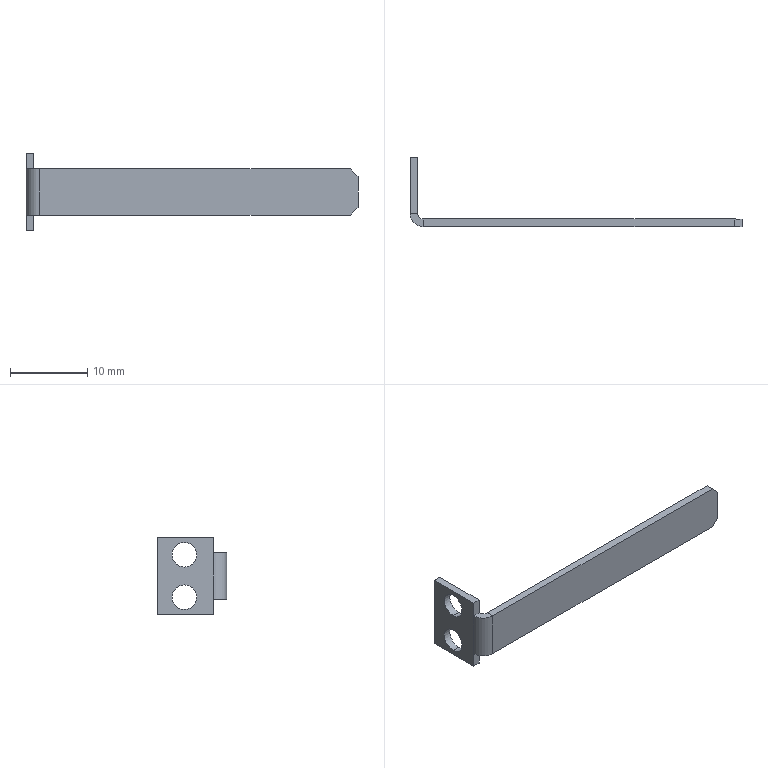Part | STEP file | lead screw origin sensing plate | 1 solid | 22 faces | box 43 x 9 x 10 mm | volume 314.784 mm3 | plane 16 | cylinder 6 | commonest cylinder face diameters 3.2 x4 1.473 x1 3.473 x1
STEP:
#1=CARTESIAN_POINT('',(0.,0.,0.));
#2=DIRECTION('',(0.,0.,1.));
#3=DIRECTION('',(1.,0.,0.));
#4=AXIS2_PLACEMENT_3D('',#1,#2,#3);
#5=CARTESIAN_POINT('',(-1.,4.5,6.15));
#6=VERTEX_POINT('',#5);
#7=CARTESIAN_POINT('',(0.,4.5,6.15));
#8=VERTEX_POINT('',#7);
#9=CARTESIAN_POINT('',(0.,4.5,6.15));
#10=DIRECTION('',(1.,0.,0.));
#11=VECTOR('',#10,1.);
#12=LINE('',#9,#11);
#13=CARTESIAN_POINT('',(0.,4.5,7.75));
#14=DIRECTION('',(1.,0.,0.));
#15=DIRECTION('',(0.,0.,-1.));
#16=AXIS2_PLACEMENT_3D('',#13,#14,#15);
#17=CYLINDRICAL_SURFACE('',#16,1.6);
#18=CARTESIAN_POINT('',(6.283,0.));
#19=DIRECTION('',(0.,1.));
#20=VECTOR('',#19,1.);
#21=LINE('',#18,#20);
#22=(GEOMETRIC_REPRESENTATION_CONTEXT(2)PARAMETRIC_REPRESENTATION_CONTEXT()REPRESENTATION_CONTEXT('',''));
#23=DEFINITIONAL_REPRESENTATION('',(#21),#22);
#24=PCURVE('',#17,#23);
#25=CARTESIAN_POINT('',(0.,4.5,7.75));
#26=DIRECTION('',(1.,0.,0.));
#27=DIRECTION('',(0.,0.,-1.));
#28=AXIS2_PLACEMENT_3D('',#25,#26,#27);
#29=CYLINDRICAL_SURFACE('',#28,1.6);
#30=CARTESIAN_POINT('',(0.,0.));
#31=DIRECTION('',(0.,1.));
#32=VECTOR('',#31,1.);
#33=LINE('',#30,#32);
#34=(GEOMETRIC_REPRESENTATION_CONTEXT(2)PARAMETRIC_REPRESENTATION_CONTEXT()REPRESENTATION_CONTEXT('',''));
#35=DEFINITIONAL_REPRESENTATION('',(#33),#34);
#36=PCURVE('',#29,#35);
#37=SURFACE_CURVE('',#12,(#24,#36),.PCURVE_S1.);
#38=EDGE_CURVE('',#6,#8,#37,.T.);
#39=ORIENTED_EDGE('',*,*,#38,.T.);
#40=CARTESIAN_POINT('',(0.,4.5,9.35));
#41=VERTEX_POINT('',#40);
#42=CARTESIAN_POINT('',(0.,4.5,7.75));
#43=DIRECTION('',(1.,0.,0.));
#44=DIRECTION('',(0.,0.,-1.));
#45=AXIS2_PLACEMENT_3D('',#42,#43,#44);
#46=CIRCLE('',#45,1.6);
#47=CARTESIAN_POINT('',(0.,0.));
#48=DIRECTION('',(1.,0.));
#49=VECTOR('',#48,1.);
#50=LINE('',#47,#49);
#51=(GEOMETRIC_REPRESENTATION_CONTEXT(2)PARAMETRIC_REPRESENTATION_CONTEXT()REPRESENTATION_CONTEXT('',''));
#52=DEFINITIONAL_REPRESENTATION('',(#50),#51);
#53=PCURVE('',#17,#52);
#54=CARTESIAN_POINT('',(0.,8.,10.));
#55=DIRECTION('',(1.,0.,0.));
#56=DIRECTION('',(0.,0.,-1.));
#57=AXIS2_PLACEMENT_3D('',#54,#55,#56);
#58=PLANE('',#57);
#59=CARTESIAN_POINT('',(2.25,-3.5));
#60=DIRECTION('',(1.,0.));
#61=AXIS2_PLACEMENT_2D('',#59,#60);
#62=CIRCLE('',#61,1.6);
#63=(GEOMETRIC_REPRESENTATION_CONTEXT(2)PARAMETRIC_REPRESENTATION_CONTEXT()REPRESENTATION_CONTEXT('',''));
#64=DEFINITIONAL_REPRESENTATION('',(#62),#63);
#65=PCURVE('',#58,#64);
#66=SURFACE_CURVE('',#46,(#53,#65),.PCURVE_S1.);
#67=EDGE_CURVE('',#41,#8,#66,.T.);
#68=ORIENTED_EDGE('',*,*,#67,.F.);
#69=CARTESIAN_POINT('',(-1.,4.5,9.35));
#70=VERTEX_POINT('',#69);
#71=CARTESIAN_POINT('',(0.,4.5,9.35));
#72=DIRECTION('',(1.,0.,0.));
#73=VECTOR('',#72,1.);
#74=LINE('',#71,#73);
#75=CARTESIAN_POINT('',(3.142,0.));
#76=DIRECTION('',(0.,1.));
#77=VECTOR('',#76,1.);
#78=LINE('',#75,#77);
#79=(GEOMETRIC_REPRESENTATION_CONTEXT(2)PARAMETRIC_REPRESENTATION_CONTEXT()REPRESENTATION_CONTEXT('',''));
#80=DEFINITIONAL_REPRESENTATION('',(#78),#79);
#81=PCURVE('',#17,#80);
#82=CARTESIAN_POINT('',(3.142,0.));
#83=DIRECTION('',(0.,1.));
#84=VECTOR('',#83,1.);
#85=LINE('',#82,#84);
#86=(GEOMETRIC_REPRESENTATION_CONTEXT(2)PARAMETRIC_REPRESENTATION_CONTEXT()REPRESENTATION_CONTEXT('',''));
#87=DEFINITIONAL_REPRESENTATION('',(#85),#86);
#88=PCURVE('',#29,#87);
#89=SURFACE_CURVE('',#74,(#81,#88),.PCURVE_S1.);
#90=EDGE_CURVE('',#70,#41,#89,.T.);
#91=ORIENTED_EDGE('',*,*,#90,.F.);
#92=CARTESIAN_POINT('',(-1.,4.5,7.75));
#93=DIRECTION('',(1.,0.,0.));
#94=DIRECTION('',(0.,0.,-1.));
#95=AXIS2_PLACEMENT_3D('',#92,#93,#94);
#96=CIRCLE('',#95,1.6);
#97=CARTESIAN_POINT('',(0.,-1.));
#98=DIRECTION('',(1.,0.));
#99=VECTOR('',#98,1.);
#100=LINE('',#97,#99);
#101=(GEOMETRIC_REPRESENTATION_CONTEXT(2)PARAMETRIC_REPRESENTATION_CONTEXT()REPRESENTATION_CONTEXT('',''));
#102=DEFINITIONAL_REPRESENTATION('',(#100),#101);
#103=PCURVE('',#17,#102);
#104=CARTESIAN_POINT('',(-1.,8.,10.));
#105=DIRECTION('',(1.,0.,0.));
#106=DIRECTION('',(0.,0.,-1.));
#107=AXIS2_PLACEMENT_3D('',#104,#105,#106);
#108=PLANE('',#107);
#109=CARTESIAN_POINT('',(2.25,-3.5));
#110=DIRECTION('',(1.,0.));
#111=AXIS2_PLACEMENT_2D('',#109,#110);
#112=CIRCLE('',#111,1.6);
#113=(GEOMETRIC_REPRESENTATION_CONTEXT(2)PARAMETRIC_REPRESENTATION_CONTEXT()REPRESENTATION_CONTEXT('',''));
#114=DEFINITIONAL_REPRESENTATION('',(#112),#113);
#115=PCURVE('',#108,#114);
#116=SURFACE_CURVE('',#96,(#103,#115),.PCURVE_S1.);
#117=EDGE_CURVE('',#70,#6,#116,.T.);
#118=ORIENTED_EDGE('',*,*,#117,.T.);
#119=EDGE_LOOP('',(#39,#68,#91,#118));
#120=FACE_BOUND('',#119,.F.);
#121=ADVANCED_FACE('',(#120),#17,.F.);
#122=CARTESIAN_POINT('',(-1.,4.5,0.65));
#123=VERTEX_POINT('',#122);
#124=CARTESIAN_POINT('',(0.,4.5,0.65));
#125=VERTEX_POINT('',#124);
#126=CARTESIAN_POINT('',(0.,4.5,0.65));
#127=DIRECTION('',(1.,0.,0.));
#128=VECTOR('',#127,1.);
#129=LINE('',#126,#128);
#130=CARTESIAN_POINT('',(0.,4.5,2.25));
#131=DIRECTION('',(1.,0.,0.));
#132=DIRECTION('',(0.,0.,-1.));
#133=AXIS2_PLACEMENT_3D('',#130,#131,#132);
#134=CYLINDRICAL_SURFACE('',#133,1.6);
#135=CARTESIAN_POINT('',(6.283,0.));
#136=DIRECTION('',(0.,1.));
#137=VECTOR('',#136,1.);
#138=LINE('',#135,#137);
#139=(GEOMETRIC_REPRESENTATION_CONTEXT(2)PARAMETRIC_REPRESENTATION_CONTEXT()REPRESENTATION_CONTEXT('',''));
#140=DEFINITIONAL_REPRESENTATION('',(#138),#139);
#141=PCURVE('',#134,#140);
#142=CARTESIAN_POINT('',(0.,4.5,2.25));
#143=DIRECTION('',(1.,0.,0.));
#144=DIRECTION('',(0.,0.,-1.));
#145=AXIS2_PLACEMENT_3D('',#142,#143,#144);
#146=CYLINDRICAL_SURFACE('',#145,1.6);
#147=CARTESIAN_POINT('',(0.,0.));
#148=DIRECTION('',(0.,1.));
#149=VECTOR('',#148,1.);
#150=LINE('',#147,#149);
#151=(GEOMETRIC_REPRESENTATION_CONTEXT(2)PARAMETRIC_REPRESENTATION_CONTEXT()REPRESENTATION_CONTEXT('',''));
#152=DEFINITIONAL_REPRESENTATION('',(#150),#151);
#153=PCURVE('',#146,#152);
#154=SURFACE_CURVE('',#129,(#141,#153),.PCURVE_S1.);
#155=EDGE_CURVE('',#123,#125,#154,.T.);
#156=ORIENTED_EDGE('',*,*,#155,.T.);
#157=CARTESIAN_POINT('',(0.,4.5,3.85));
#158=VERTEX_POINT('',#157);
#159=CARTESIAN_POINT('',(0.,4.5,2.25));
#160=DIRECTION('',(1.,0.,0.));
#161=DIRECTION('',(0.,0.,-1.));
#162=AXIS2_PLACEMENT_3D('',#159,#160,#161);
#163=CIRCLE('',#162,1.6);
#164=CARTESIAN_POINT('',(0.,0.));
#165=DIRECTION('',(1.,0.));
#166=VECTOR('',#165,1.);
#167=LINE('',#164,#166);
#168=(GEOMETRIC_REPRESENTATION_CONTEXT(2)PARAMETRIC_REPRESENTATION_CONTEXT()REPRESENTATION_CONTEXT('',''));
#169=DEFINITIONAL_REPRESENTATION('',(#167),#168);
#170=PCURVE('',#134,#169);
#171=CARTESIAN_POINT('',(7.75,-3.5));
#172=DIRECTION('',(1.,0.));
#173=AXIS2_PLACEMENT_2D('',#171,#172);
#174=CIRCLE('',#173,1.6);
#175=(GEOMETRIC_REPRESENTATION_CONTEXT(2)PARAMETRIC_REPRESENTATION_CONTEXT()REPRESENTATION_CONTEXT('',''));
#176=DEFINITIONAL_REPRESENTATION('',(#174),#175);
#177=PCURVE('',#58,#176);
#178=SURFACE_CURVE('',#163,(#170,#177),.PCURVE_S1.);
#179=EDGE_CURVE('',#158,#125,#178,.T.);
#180=ORIENTED_EDGE('',*,*,#179,.F.);
#181=CARTESIAN_POINT('',(-1.,4.5,3.85));
#182=VERTEX_POINT('',#181);
#183=CARTESIAN_POINT('',(0.,4.5,3.85));
#184=DIRECTION('',(1.,0.,0.));
#185=VECTOR('',#184,1.);
#186=LINE('',#183,#185);
#187=CARTESIAN_POINT('',(3.142,0.));
#188=DIRECTION('',(0.,1.));
#189=VECTOR('',#188,1.);
#190=LINE('',#187,#189);
#191=(GEOMETRIC_REPRESENTATION_CONTEXT(2)PARAMETRIC_REPRESENTATION_CONTEXT()REPRESENTATION_CONTEXT('',''));
#192=DEFINITIONAL_REPRESENTATION('',(#190),#191);
#193=PCURVE('',#134,#192);
#194=CARTESIAN_POINT('',(3.142,0.));
#195=DIRECTION('',(0.,1.));
#196=VECTOR('',#195,1.);
#197=LINE('',#194,#196);
#198=(GEOMETRIC_REPRESENTATION_CONTEXT(2)PARAMETRIC_REPRESENTATION_CONTEXT()REPRESENTATION_CONTEXT('',''));
#199=DEFINITIONAL_REPRESENTATION('',(#197),#198);
#200=PCURVE('',#146,#199);
#201=SURFACE_CURVE('',#186,(#193,#200),.PCURVE_S1.);
#202=EDGE_CURVE('',#182,#158,#201,.T.);
#203=ORIENTED_EDGE('',*,*,#202,.F.);
#204=CARTESIAN_POINT('',(-1.,4.5,2.25));
#205=DIRECTION('',(1.,0.,0.));
#206=DIRECTION('',(0.,0.,-1.));
#207=AXIS2_PLACEMENT_3D('',#204,#205,#206);
#208=CIRCLE('',#207,1.6);
#209=CARTESIAN_POINT('',(0.,-1.));
#210=DIRECTION('',(1.,0.));
#211=VECTOR('',#210,1.);
#212=LINE('',#209,#211);
#213=(GEOMETRIC_REPRESENTATION_CONTEXT(2)PARAMETRIC_REPRESENTATION_CONTEXT()REPRESENTATION_CONTEXT('',''));
#214=DEFINITIONAL_REPRESENTATION('',(#212),#213);
#215=PCURVE('',#134,#214);
#216=CARTESIAN_POINT('',(7.75,-3.5));
#217=DIRECTION('',(1.,0.));
#218=AXIS2_PLACEMENT_2D('',#216,#217);
#219=CIRCLE('',#218,1.6);
#220=(GEOMETRIC_REPRESENTATION_CONTEXT(2)PARAMETRIC_REPRESENTATION_CONTEXT()REPRESENTATION_CONTEXT('',''));
#221=DEFINITIONAL_REPRESENTATION('',(#219),#220);
#222=PCURVE('',#108,#221);
#223=SURFACE_CURVE('',#208,(#215,#222),.PCURVE_S1.);
#224=EDGE_CURVE('',#182,#123,#223,.T.);
#225=ORIENTED_EDGE('',*,*,#224,.T.);
#226=EDGE_LOOP('',(#156,#180,#203,#225));
#227=FACE_BOUND('',#226,.F.);
#228=ADVANCED_FACE('',(#227),#134,.F.);
#229=CARTESIAN_POINT('',(0.7366,0.,2.));
#230=VERTEX_POINT('',#229);
#231=CARTESIAN_POINT('',(0.,0.7366,2.));
#232=VERTEX_POINT('',#231);
#233=CARTESIAN_POINT('',(0.7366,0.7366,2.));
#234=DIRECTION('',(0.,0.,-1.));
#235=DIRECTION('',(-1.,0.,0.));
#236=AXIS2_PLACEMENT_3D('',#233,#234,#235);
#237=CIRCLE('',#236,0.7366);
#238=CARTESIAN_POINT('',(0.7366,0.7366,10.));
#239=DIRECTION('',(0.,0.,-1.));
#240=DIRECTION('',(-1.,0.,0.));
#241=AXIS2_PLACEMENT_3D('',#238,#239,#240);
#242=CYLINDRICAL_SURFACE('',#241,0.7366);
#243=CARTESIAN_POINT('',(0.,8.));
#244=DIRECTION('',(1.,0.));
#245=VECTOR('',#244,1.);
#246=LINE('',#243,#245);
#247=(GEOMETRIC_REPRESENTATION_CONTEXT(2)PARAMETRIC_REPRESENTATION_CONTEXT()REPRESENTATION_CONTEXT('',''));
#248=DEFINITIONAL_REPRESENTATION('',(#246),#247);
#249=PCURVE('',#242,#248);
#250=CARTESIAN_POINT('',(0.7366,0.7366,2.));
#251=DIRECTION('',(0.,0.,-1.));
#252=DIRECTION('',(-1.,0.,0.));
#253=AXIS2_PLACEMENT_3D('',#250,#251,#252);
#254=PLANE('',#253);
#255=CARTESIAN_POINT('',(0.,0.));
#256=DIRECTION('',(1.,0.));
#257=AXIS2_PLACEMENT_2D('',#255,#256);
#258=CIRCLE('',#257,0.7366);
#259=(GEOMETRIC_REPRESENTATION_CONTEXT(2)PARAMETRIC_REPRESENTATION_CONTEXT()REPRESENTATION_CONTEXT('',''));
#260=DEFINITIONAL_REPRESENTATION('',(#258),#259);
#261=PCURVE('',#254,#260);
#262=SURFACE_CURVE('',#237,(#249,#261),.PCURVE_S1.);
#263=EDGE_CURVE('',#230,#232,#262,.T.);
#264=ORIENTED_EDGE('',*,*,#263,.F.);
#265=CARTESIAN_POINT('',(0.7366,0.,8.));
#266=VERTEX_POINT('',#265);
#267=CARTESIAN_POINT('',(0.7366,0.,10.));
#268=DIRECTION('',(0.,0.,-1.));
#269=VECTOR('',#268,1.);
#270=LINE('',#267,#269);
#271=CARTESIAN_POINT('',(4.712,0.));
#272=DIRECTION('',(0.,1.));
#273=VECTOR('',#272,1.);
#274=LINE('',#271,#273);
#275=(GEOMETRIC_REPRESENTATION_CONTEXT(2)PARAMETRIC_REPRESENTATION_CONTEXT()REPRESENTATION_CONTEXT('',''));
#276=DEFINITIONAL_REPRESENTATION('',(#274),#275);
#277=PCURVE('',#242,#276);
#278=CARTESIAN_POINT('',(0.,0.,10.));
#279=DIRECTION('',(0.,1.,0.));
#280=DIRECTION('',(0.,0.,1.));
#281=AXIS2_PLACEMENT_3D('',#278,#279,#280);
#282=PLANE('',#281);
#283=CARTESIAN_POINT('',(0.,0.7366));
#284=DIRECTION('',(-1.,0.));
#285=VECTOR('',#284,1.);
#286=LINE('',#283,#285);
#287=(GEOMETRIC_REPRESENTATION_CONTEXT(2)PARAMETRIC_REPRESENTATION_CONTEXT()REPRESENTATION_CONTEXT('',''));
#288=DEFINITIONAL_REPRESENTATION('',(#286),#287);
#289=PCURVE('',#282,#288);
#290=SURFACE_CURVE('',#270,(#277,#289),.PCURVE_S1.);
#291=EDGE_CURVE('',#266,#230,#290,.T.);
#292=ORIENTED_EDGE('',*,*,#291,.F.);
#293=CARTESIAN_POINT('',(0.,0.7366,8.));
#294=VERTEX_POINT('',#293);
#295=CARTESIAN_POINT('',(0.7366,0.7366,8.));
#296=DIRECTION('',(0.,0.,-1.));
#297=DIRECTION('',(-1.,0.,0.));
#298=AXIS2_PLACEMENT_3D('',#295,#296,#297);
#299=CIRCLE('',#298,0.7366);
#300=CARTESIAN_POINT('',(0.,2.));
#301=DIRECTION('',(1.,0.));
#302=VECTOR('',#301,1.);
#303=LINE('',#300,#302);
#304=(GEOMETRIC_REPRESENTATION_CONTEXT(2)PARAMETRIC_REPRESENTATION_CONTEXT()REPRESENTATION_CONTEXT('',''));
#305=DEFINITIONAL_REPRESENTATION('',(#303),#304);
#306=PCURVE('',#242,#305);
#307=CARTESIAN_POINT('',(0.7366,0.7366,8.));
#308=DIRECTION('',(0.,0.,1.));
#309=DIRECTION('',(1.,0.,0.));
#310=AXIS2_PLACEMENT_3D('',#307,#308,#309);
#311=PLANE('',#310);
#312=CARTESIAN_POINT('',(-0.7366,0.));
#313=CARTESIAN_POINT('',(-0.7366,1.276));
#314=CARTESIAN_POINT('',(0.3683,0.6379));
#315=CARTESIAN_POINT('',(1.473,0.));
#316=CARTESIAN_POINT('',(0.3683,-0.6379));
#317=CARTESIAN_POINT('',(-0.7366,-1.276));
#318=CARTESIAN_POINT('',(-0.7366,0.));
#319=(BOUNDED_CURVE()B_SPLINE_CURVE(2,(#312,#313,#314,#315,#316,#317,#318),.UNSPECIFIED.,.T.,.F.)B_SPLINE_CURVE_WITH_KNOTS((1,2,2,2,2,1),(-2.094,0.,2.094,4.189,6.283,8.378),.UNSPECIFIED.)CURVE()GEOMETRIC_REPRESENTATION_ITEM()RATIONAL_B_SPLINE_CURVE((1.,0.5,1.,0.5,1.,0.5,1.))REPRESENTATION_ITEM(''));
#320=(GEOMETRIC_REPRESENTATION_CONTEXT(2)PARAMETRIC_REPRESENTATION_CONTEXT()REPRESENTATION_CONTEXT('',''));
#321=DEFINITIONAL_REPRESENTATION('',(#319),#320);
#322=PCURVE('',#311,#321);
#323=SURFACE_CURVE('',#299,(#306,#322),.PCURVE_S1.);
#324=EDGE_CURVE('',#266,#294,#323,.T.);
#325=ORIENTED_EDGE('',*,*,#324,.T.);
#326=CARTESIAN_POINT('',(0.,0.7366,10.));
#327=DIRECTION('',(0.,0.,-1.));
#328=VECTOR('',#327,1.);
#329=LINE('',#326,#328);
#330=CARTESIAN_POINT('',(6.283,0.));
#331=DIRECTION('',(0.,1.));
#332=VECTOR('',#331,1.);
#333=LINE('',#330,#332);
#334=(GEOMETRIC_REPRESENTATION_CONTEXT(2)PARAMETRIC_REPRESENTATION_CONTEXT()REPRESENTATION_CONTEXT('',''));
#335=DEFINITIONAL_REPRESENTATION('',(#333),#334);
#336=PCURVE('',#242,#335);
#337=CARTESIAN_POINT('',(0.,-7.263));
#338=DIRECTION('',(1.,0.));
#339=VECTOR('',#338,1.);
#340=LINE('',#337,#339);
#341=(GEOMETRIC_REPRESENTATION_CONTEXT(2)PARAMETRIC_REPRESENTATION_CONTEXT()REPRESENTATION_CONTEXT('',''));
#342=DEFINITIONAL_REPRESENTATION('',(#340),#341);
#343=PCURVE('',#58,#342);
#344=SURFACE_CURVE('',#329,(#336,#343),.PCURVE_S1.);
#345=EDGE_CURVE('',#294,#232,#344,.T.);
#346=ORIENTED_EDGE('',*,*,#345,.T.);
#347=EDGE_LOOP('',(#264,#292,#325,#346));
#348=FACE_BOUND('',#347,.F.);
#349=ADVANCED_FACE('',(#348),#242,.F.);
#350=CARTESIAN_POINT('',(0.7366,-1.,8.));
#351=VERTEX_POINT('',#350);
#352=CARTESIAN_POINT('',(-1.,0.7366,8.));
#353=VERTEX_POINT('',#352);
#354=CARTESIAN_POINT('',(0.7366,0.7366,8.));
#355=DIRECTION('',(0.,0.,-1.));
#356=DIRECTION('',(-1.,0.,0.));
#357=AXIS2_PLACEMENT_3D('',#354,#355,#356);
#358=CIRCLE('',#357,1.737);
#359=CARTESIAN_POINT('',(0.7366,0.7366,10.));
#360=DIRECTION('',(0.,0.,-1.));
#361=DIRECTION('',(-1.,0.,0.));
#362=AXIS2_PLACEMENT_3D('',#359,#360,#361);
#363=CYLINDRICAL_SURFACE('',#362,1.737);
#364=CARTESIAN_POINT('',(0.,2.));
#365=DIRECTION('',(1.,0.));
#366=VECTOR('',#365,1.);
#367=LINE('',#364,#366);
#368=(GEOMETRIC_REPRESENTATION_CONTEXT(2)PARAMETRIC_REPRESENTATION_CONTEXT()REPRESENTATION_CONTEXT('',''));
#369=DEFINITIONAL_REPRESENTATION('',(#367),#368);
#370=PCURVE('',#363,#369);
#371=CARTESIAN_POINT('',(-1.737,0.));
#372=CARTESIAN_POINT('',(-1.737,3.008));
#373=CARTESIAN_POINT('',(0.8683,1.504));
#374=CARTESIAN_POINT('',(3.473,0.));
#375=CARTESIAN_POINT('',(0.8683,-1.504));
#376=CARTESIAN_POINT('',(-1.737,-3.008));
#377=CARTESIAN_POINT('',(-1.737,0.));
#378=(BOUNDED_CURVE()B_SPLINE_CURVE(2,(#371,#372,#373,#374,#375,#376,#377),.UNSPECIFIED.,.T.,.F.)B_SPLINE_CURVE_WITH_KNOTS((1,2,2,2,2,1),(-2.094,0.,2.094,4.189,6.283,8.378),.UNSPECIFIED.)CURVE()GEOMETRIC_REPRESENTATION_ITEM()RATIONAL_B_SPLINE_CURVE((1.,0.5,1.,0.5,1.,0.5,1.))REPRESENTATION_ITEM(''));
#379=(GEOMETRIC_REPRESENTATION_CONTEXT(2)PARAMETRIC_REPRESENTATION_CONTEXT()REPRESENTATION_CONTEXT('',''));
#380=DEFINITIONAL_REPRESENTATION('',(#378),#379);
#381=PCURVE('',#311,#380);
#382=SURFACE_CURVE('',#358,(#370,#381),.PCURVE_S1.);
#383=EDGE_CURVE('',#351,#353,#382,.T.);
#384=ORIENTED_EDGE('',*,*,#383,.T.);
#385=CARTESIAN_POINT('',(-1.,0.7366,2.));
#386=VERTEX_POINT('',#385);
#387=CARTESIAN_POINT('',(-1.,0.7366,10.));
#388=DIRECTION('',(0.,0.,-1.));
#389=VECTOR('',#388,1.);
#390=LINE('',#387,#389);
#391=CARTESIAN_POINT('',(6.283,0.));
#392=DIRECTION('',(0.,1.));
#393=VECTOR('',#392,1.);
#394=LINE('',#391,#393);
#395=(GEOMETRIC_REPRESENTATION_CONTEXT(2)PARAMETRIC_REPRESENTATION_CONTEXT()REPRESENTATION_CONTEXT('',''));
#396=DEFINITIONAL_REPRESENTATION('',(#394),#395);
#397=PCURVE('',#363,#396);
#398=CARTESIAN_POINT('',(0.,-7.263));
#399=DIRECTION('',(1.,0.));
#400=VECTOR('',#399,1.);
#401=LINE('',#398,#400);
#402=(GEOMETRIC_REPRESENTATION_CONTEXT(2)PARAMETRIC_REPRESENTATION_CONTEXT()REPRESENTATION_CONTEXT('',''));
#403=DEFINITIONAL_REPRESENTATION('',(#401),#402);
#404=PCURVE('',#108,#403);
#405=SURFACE_CURVE('',#390,(#397,#404),.PCURVE_S1.);
#406=EDGE_CURVE('',#353,#386,#405,.T.);
#407=ORIENTED_EDGE('',*,*,#406,.T.);
#408=CARTESIAN_POINT('',(0.7366,-1.,2.));
#409=VERTEX_POINT('',#408);
#410=CARTESIAN_POINT('',(0.7366,0.7366,2.));
#411=DIRECTION('',(0.,0.,-1.));
#412=DIRECTION('',(1.,0.,0.));
#413=AXIS2_PLACEMENT_3D('',#410,#411,#412);
#414=CIRCLE('',#413,1.737);
#415=CARTESIAN_POINT('',(3.142,8.));
#416=DIRECTION('',(1.,0.));
#417=VECTOR('',#416,1.);
#418=LINE('',#415,#417);
#419=(GEOMETRIC_REPRESENTATION_CONTEXT(2)PARAMETRIC_REPRESENTATION_CONTEXT()REPRESENTATION_CONTEXT('',''));
#420=DEFINITIONAL_REPRESENTATION('',(#418),#419);
#421=PCURVE('',#363,#420);
#422=CARTESIAN_POINT('',(0.,0.));
#423=DIRECTION('',(-1.,0.));
#424=AXIS2_PLACEMENT_2D('',#422,#423);
#425=CIRCLE('',#424,1.737);
#426=(GEOMETRIC_REPRESENTATION_CONTEXT(2)PARAMETRIC_REPRESENTATION_CONTEXT()REPRESENTATION_CONTEXT('',''));
#427=DEFINITIONAL_REPRESENTATION('',(#425),#426);
#428=PCURVE('',#254,#427);
#429=SURFACE_CURVE('',#414,(#421,#428),.PCURVE_S1.);
#430=EDGE_CURVE('',#409,#386,#429,.T.);
#431=ORIENTED_EDGE('',*,*,#430,.F.);
#432=CARTESIAN_POINT('',(0.7366,-1.,10.));
#433=DIRECTION('',(0.,0.,-1.));
#434=VECTOR('',#433,1.);
#435=LINE('',#432,#434);
#436=CARTESIAN_POINT('',(4.712,0.));
#437=DIRECTION('',(0.,1.));
#438=VECTOR('',#437,1.);
#439=LINE('',#436,#438);
#440=(GEOMETRIC_REPRESENTATION_CONTEXT(2)PARAMETRIC_REPRESENTATION_CONTEXT()REPRESENTATION_CONTEXT('',''));
#441=DEFINITIONAL_REPRESENTATION('',(#439),#440);
#442=PCURVE('',#363,#441);
#443=CARTESIAN_POINT('',(0.,-1.,10.));
#444=DIRECTION('',(0.,1.,0.));
#445=DIRECTION('',(0.,0.,1.));
#446=AXIS2_PLACEMENT_3D('',#443,#444,#445);
#447=PLANE('',#446);
#448=CARTESIAN_POINT('',(0.,0.7366));
#449=DIRECTION('',(-1.,0.));
#450=VECTOR('',#449,1.);
#451=LINE('',#448,#450);
#452=(GEOMETRIC_REPRESENTATION_CONTEXT(2)PARAMETRIC_REPRESENTATION_CONTEXT()REPRESENTATION_CONTEXT('',''));
#453=DEFINITIONAL_REPRESENTATION('',(#451),#452);
#454=PCURVE('',#447,#453);
#455=SURFACE_CURVE('',#435,(#442,#454),.PCURVE_S1.);
#456=EDGE_CURVE('',#351,#409,#455,.T.);
#457=ORIENTED_EDGE('',*,*,#456,.F.);
#458=EDGE_LOOP('',(#384,#407,#431,#457));
#459=FACE_BOUND('',#458,.T.);
#460=ADVANCED_FACE('',(#459),#363,.T.);
#461=CARTESIAN_POINT('',(0.,8.,0.));
#462=VERTEX_POINT('',#461);
#463=CARTESIAN_POINT('',(0.,0.7366,0.));
#464=VERTEX_POINT('',#463);
#465=CARTESIAN_POINT('',(0.,8.,0.));
#466=DIRECTION('',(0.,-1.,0.));
#467=VECTOR('',#466,1.);
#468=LINE('',#465,#467);
#469=CARTESIAN_POINT('',(0.7366,-1.,0.));
#470=DIRECTION('',(0.,0.,-1.));
#471=DIRECTION('',(-1.,0.,0.));
#472=AXIS2_PLACEMENT_3D('',#469,#470,#471);
#473=PLANE('',#472);
#474=CARTESIAN_POINT('',(0.7366,9.));
#475=DIRECTION('',(0.,-1.));
#476=VECTOR('',#475,1.);
#477=LINE('',#474,#476);
#478=(GEOMETRIC_REPRESENTATION_CONTEXT(2)PARAMETRIC_REPRESENTATION_CONTEXT()REPRESENTATION_CONTEXT('',''));
#479=DEFINITIONAL_REPRESENTATION('',(#477),#478);
#480=PCURVE('',#473,#479);
#481=CARTESIAN_POINT('',(10.,0.));
#482=DIRECTION('',(0.,-1.));
#483=VECTOR('',#482,1.);
#484=LINE('',#481,#483);
#485=(GEOMETRIC_REPRESENTATION_CONTEXT(2)PARAMETRIC_REPRESENTATION_CONTEXT()REPRESENTATION_CONTEXT('',''));
#486=DEFINITIONAL_REPRESENTATION('',(#484),#485);
#487=PCURVE('',#58,#486);
#488=SURFACE_CURVE('',#468,(#480,#487),.PCURVE_S1.);
#489=EDGE_CURVE('',#462,#464,#488,.T.);
#490=ORIENTED_EDGE('',*,*,#489,.T.);
#491=CARTESIAN_POINT('',(-1.,0.7366,0.));
#492=VERTEX_POINT('',#491);
#493=CARTESIAN_POINT('',(0.,0.7366,0.));
#494=DIRECTION('',(-1.,0.,0.));
#495=VECTOR('',#494,1.);
#496=LINE('',#493,#495);
#497=CARTESIAN_POINT('',(0.7366,1.737));
#498=DIRECTION('',(1.,0.));
#499=VECTOR('',#498,1.);
#500=LINE('',#497,#499);
#501=(GEOMETRIC_REPRESENTATION_CONTEXT(2)PARAMETRIC_REPRESENTATION_CONTEXT()REPRESENTATION_CONTEXT('',''));
#502=DEFINITIONAL_REPRESENTATION('',(#500),#501);
#503=PCURVE('',#473,#502);
#504=CARTESIAN_POINT('',(-1.,0.7366,1.));
#505=DIRECTION('',(0.,1.,0.));
#506=DIRECTION('',(0.,0.,-1.));
#507=AXIS2_PLACEMENT_3D('',#504,#505,#506);
#508=PLANE('',#507);
#509=CARTESIAN_POINT('',(1.,-1.));
#510=DIRECTION('',(0.,1.));
#511=VECTOR('',#510,1.);
#512=LINE('',#509,#511);
#513=(GEOMETRIC_REPRESENTATION_CONTEXT(2)PARAMETRIC_REPRESENTATION_CONTEXT()REPRESENTATION_CONTEXT('',''));
#514=DEFINITIONAL_REPRESENTATION('',(#512),#513);
#515=PCURVE('',#508,#514);
#516=SURFACE_CURVE('',#496,(#503,#515),.PCURVE_S1.);
#517=EDGE_CURVE('',#464,#492,#516,.T.);
#518=ORIENTED_EDGE('',*,*,#517,.T.);
#519=CARTESIAN_POINT('',(-1.,8.,0.));
#520=VERTEX_POINT('',#519);
#521=CARTESIAN_POINT('',(-1.,8.,0.));
#522=DIRECTION('',(0.,-1.,0.));
#523=VECTOR('',#522,1.);
#524=LINE('',#521,#523);
#525=CARTESIAN_POINT('',(1.737,9.));
#526=DIRECTION('',(0.,-1.));
#527=VECTOR('',#526,1.);
#528=LINE('',#525,#527);
#529=(GEOMETRIC_REPRESENTATION_CONTEXT(2)PARAMETRIC_REPRESENTATION_CONTEXT()REPRESENTATION_CONTEXT('',''));
#530=DEFINITIONAL_REPRESENTATION('',(#528),#529);
#531=PCURVE('',#473,#530);
#532=CARTESIAN_POINT('',(10.,0.));
#533=DIRECTION('',(0.,-1.));
#534=VECTOR('',#533,1.);
#535=LINE('',#532,#534);
#536=(GEOMETRIC_REPRESENTATION_CONTEXT(2)PARAMETRIC_REPRESENTATION_CONTEXT()REPRESENTATION_CONTEXT('',''));
#537=DEFINITIONAL_REPRESENTATION('',(#535),#536);
#538=PCURVE('',#108,#537);
#539=SURFACE_CURVE('',#524,(#531,#538),.PCURVE_S1.);
#540=EDGE_CURVE('',#520,#492,#539,.T.);
#541=ORIENTED_EDGE('',*,*,#540,.F.);
#542=CARTESIAN_POINT('',(-1.,8.,0.));
#543=DIRECTION('',(1.,0.,0.));
#544=VECTOR('',#543,1.);
#545=LINE('',#542,#544);
#546=CARTESIAN_POINT('',(1.737,9.));
#547=DIRECTION('',(-1.,0.));
#548=VECTOR('',#547,1.);
#549=LINE('',#546,#548);
#550=(GEOMETRIC_REPRESENTATION_CONTEXT(2)PARAMETRIC_REPRESENTATION_CONTEXT()REPRESENTATION_CONTEXT('',''));
#551=DEFINITIONAL_REPRESENTATION('',(#549),#550);
#552=PCURVE('',#473,#551);
#553=CARTESIAN_POINT('',(-1.,8.,10.));
#554=DIRECTION('',(0.,1.,0.));
#555=DIRECTION('',(0.,0.,1.));
#556=AXIS2_PLACEMENT_3D('',#553,#554,#555);
#557=PLANE('',#556);
#558=CARTESIAN_POINT('',(-10.,0.));
#559=DIRECTION('',(0.,1.));
#560=VECTOR('',#559,1.);
#561=LINE('',#558,#560);
#562=(GEOMETRIC_REPRESENTATION_CONTEXT(2)PARAMETRIC_REPRESENTATION_CONTEXT()REPRESENTATION_CONTEXT('',''));
#563=DEFINITIONAL_REPRESENTATION('',(#561),#562);
#564=PCURVE('',#557,#563);
#565=SURFACE_CURVE('',#545,(#552,#564),.PCURVE_S1.);
#566=EDGE_CURVE('',#520,#462,#565,.T.);
#567=ORIENTED_EDGE('',*,*,#566,.T.);
#568=EDGE_LOOP('',(#490,#518,#541,#567));
#569=FACE_BOUND('',#568,.T.);
#570=ADVANCED_FACE('',(#569),#473,.T.);
#571=CARTESIAN_POINT('',(41.,-1.,2.));
#572=VERTEX_POINT('',#571);
#573=CARTESIAN_POINT('',(0.7366,-1.,2.));
#574=DIRECTION('',(1.,0.,0.));
#575=VECTOR('',#574,1.);
#576=LINE('',#573,#575);
#577=CARTESIAN_POINT('',(-8.,0.7366));
#578=DIRECTION('',(0.,1.));
#579=VECTOR('',#578,1.);
#580=LINE('',#577,#579);
#581=(GEOMETRIC_REPRESENTATION_CONTEXT(2)PARAMETRIC_REPRESENTATION_CONTEXT()REPRESENTATION_CONTEXT('',''));
#582=DEFINITIONAL_REPRESENTATION('',(#580),#581);
#583=PCURVE('',#447,#582);
#584=CARTESIAN_POINT('',(0.7366,-1.,2.));
#585=DIRECTION('',(0.,0.,1.));
#586=DIRECTION('',(1.,0.,0.));
#587=AXIS2_PLACEMENT_3D('',#584,#585,#586);
#588=PLANE('',#587);
#589=CARTESIAN_POINT('',(0.,0.));
#590=DIRECTION('',(1.,0.));
#591=VECTOR('',#590,1.);
#592=LINE('',#589,#591);
#593=(GEOMETRIC_REPRESENTATION_CONTEXT(2)PARAMETRIC_REPRESENTATION_CONTEXT()REPRESENTATION_CONTEXT('',''));
#594=DEFINITIONAL_REPRESENTATION('',(#592),#593);
#595=PCURVE('',#588,#594);
#596=SURFACE_CURVE('',#576,(#583,#595),.PCURVE_S1.);
#597=EDGE_CURVE('',#409,#572,#596,.T.);
#598=ORIENTED_EDGE('',*,*,#597,.T.);
#599=CARTESIAN_POINT('',(42.,-1.,3.));
#600=VERTEX_POINT('',#599);
#601=CARTESIAN_POINT('',(42.,-1.,3.));
#602=DIRECTION('',(0.7071,0.,0.7071));
#603=VECTOR('',#602,1.);
#604=LINE('',#601,#603);
#605=CARTESIAN_POINT('',(-7.,42.));
#606=DIRECTION('',(0.7071,0.7071));
#607=VECTOR('',#606,1.);
#608=LINE('',#605,#607);
#609=(GEOMETRIC_REPRESENTATION_CONTEXT(2)PARAMETRIC_REPRESENTATION_CONTEXT()REPRESENTATION_CONTEXT('',''));
#610=DEFINITIONAL_REPRESENTATION('',(#608),#609);
#611=PCURVE('',#447,#610);
#612=CARTESIAN_POINT('',(42.,0.,3.));
#613=DIRECTION('',(0.7071,0.,-0.7071));
#614=DIRECTION('',(0.,-1.,0.));
#615=AXIS2_PLACEMENT_3D('',#612,#613,#614);
#616=PLANE('',#615);
#617=CARTESIAN_POINT('',(1.,0.));
#618=DIRECTION('',(0.,-1.));
#619=VECTOR('',#618,1.);
#620=LINE('',#617,#619);
#621=(GEOMETRIC_REPRESENTATION_CONTEXT(2)PARAMETRIC_REPRESENTATION_CONTEXT()REPRESENTATION_CONTEXT('',''));
#622=DEFINITIONAL_REPRESENTATION('',(#620),#621);
#623=PCURVE('',#616,#622);
#624=SURFACE_CURVE('',#604,(#611,#623),.PCURVE_S1.);
#625=EDGE_CURVE('',#572,#600,#624,.T.);
#626=ORIENTED_EDGE('',*,*,#625,.T.);
#627=CARTESIAN_POINT('',(42.,-1.,7.));
#628=VERTEX_POINT('',#627);
#629=CARTESIAN_POINT('',(42.,-1.,10.));
#630=DIRECTION('',(0.,0.,-1.));
#631=VECTOR('',#630,1.);
#632=LINE('',#629,#631);
#633=CARTESIAN_POINT('',(0.,42.));
#634=DIRECTION('',(-1.,0.));
#635=VECTOR('',#634,1.);
#636=LINE('',#633,#635);
#637=(GEOMETRIC_REPRESENTATION_CONTEXT(2)PARAMETRIC_REPRESENTATION_CONTEXT()REPRESENTATION_CONTEXT('',''));
#638=DEFINITIONAL_REPRESENTATION('',(#636),#637);
#639=PCURVE('',#447,#638);
#640=CARTESIAN_POINT('',(42.,0.,10.));
#641=DIRECTION('',(1.,0.,0.));
#642=DIRECTION('',(0.,0.,-1.));
#643=AXIS2_PLACEMENT_3D('',#640,#641,#642);
#644=PLANE('',#643);
#645=CARTESIAN_POINT('',(0.,-1.));
#646=DIRECTION('',(1.,0.));
#647=VECTOR('',#646,1.);
#648=LINE('',#645,#647);
#649=(GEOMETRIC_REPRESENTATION_CONTEXT(2)PARAMETRIC_REPRESENTATION_CONTEXT()REPRESENTATION_CONTEXT('',''));
#650=DEFINITIONAL_REPRESENTATION('',(#648),#649);
#651=PCURVE('',#644,#650);
#652=SURFACE_CURVE('',#632,(#639,#651),.PCURVE_S1.);
#653=EDGE_CURVE('',#628,#600,#652,.T.);
#654=ORIENTED_EDGE('',*,*,#653,.F.);
#655=CARTESIAN_POINT('',(41.,-1.,8.));
#656=VERTEX_POINT('',#655);
#657=CARTESIAN_POINT('',(41.,-1.,8.));
#658=DIRECTION('',(-0.7071,0.,0.7071));
#659=VECTOR('',#658,1.);
#660=LINE('',#657,#659);
#661=CARTESIAN_POINT('',(-2.,41.));
#662=DIRECTION('',(0.7071,-0.7071));
#663=VECTOR('',#662,1.);
#664=LINE('',#661,#663);
#665=(GEOMETRIC_REPRESENTATION_CONTEXT(2)PARAMETRIC_REPRESENTATION_CONTEXT()REPRESENTATION_CONTEXT('',''));
#666=DEFINITIONAL_REPRESENTATION('',(#664),#665);
#667=PCURVE('',#447,#666);
#668=CARTESIAN_POINT('',(41.,-1.,8.));
#669=DIRECTION('',(0.7071,0.,0.7071));
#670=DIRECTION('',(0.,-1.,0.));
#671=AXIS2_PLACEMENT_3D('',#668,#669,#670);
#672=PLANE('',#671);
#673=CARTESIAN_POINT('',(0.,0.));
#674=DIRECTION('',(0.,-1.));
#675=VECTOR('',#674,1.);
#676=LINE('',#673,#675);
#677=(GEOMETRIC_REPRESENTATION_CONTEXT(2)PARAMETRIC_REPRESENTATION_CONTEXT()REPRESENTATION_CONTEXT('',''));
#678=DEFINITIONAL_REPRESENTATION('',(#676),#677);
#679=PCURVE('',#672,#678);
#680=SURFACE_CURVE('',#660,(#667,#679),.PCURVE_S1.);
#681=EDGE_CURVE('',#628,#656,#680,.T.);
#682=ORIENTED_EDGE('',*,*,#681,.T.);
#683=CARTESIAN_POINT('',(0.7366,-1.,8.));
#684=DIRECTION('',(-1.,0.,0.));
#685=VECTOR('',#684,1.);
#686=LINE('',#683,#685);
#687=CARTESIAN_POINT('',(-2.,0.7366));
#688=DIRECTION('',(0.,-1.));
#689=VECTOR('',#688,1.);
#690=LINE('',#687,#689);
#691=(GEOMETRIC_REPRESENTATION_CONTEXT(2)PARAMETRIC_REPRESENTATION_CONTEXT()REPRESENTATION_CONTEXT('',''));
#692=DEFINITIONAL_REPRESENTATION('',(#690),#691);
#693=PCURVE('',#447,#692);
#694=CARTESIAN_POINT('',(0.7366,-1.,8.));
#695=DIRECTION('',(0.,0.,-1.));
#696=DIRECTION('',(-1.,0.,0.));
#697=AXIS2_PLACEMENT_3D('',#694,#695,#696);
#698=PLANE('',#697);
#699=CARTESIAN_POINT('',(0.,0.));
#700=DIRECTION('',(1.,0.));
#701=VECTOR('',#700,1.);
#702=LINE('',#699,#701);
#703=(GEOMETRIC_REPRESENTATION_CONTEXT(2)PARAMETRIC_REPRESENTATION_CONTEXT()REPRESENTATION_CONTEXT('',''));
#704=DEFINITIONAL_REPRESENTATION('',(#702),#703);
#705=PCURVE('',#698,#704);
#706=SURFACE_CURVE('',#686,(#693,#705),.PCURVE_S1.);
#707=EDGE_CURVE('',#656,#351,#706,.T.);
#708=ORIENTED_EDGE('',*,*,#707,.T.);
#709=ORIENTED_EDGE('',*,*,#456,.T.);
#710=EDGE_LOOP('',(#598,#626,#654,#682,#708,#709));
#711=FACE_BOUND('',#710,.T.);
#712=ADVANCED_FACE('',(#711),#447,.F.);
#713=ORIENTED_EDGE('',*,*,#653,.T.);
#714=CARTESIAN_POINT('',(42.,0.,3.));
#715=VERTEX_POINT('',#714);
#716=CARTESIAN_POINT('',(42.,0.,3.));
#717=DIRECTION('',(0.,1.,0.));
#718=VECTOR('',#717,1.);
#719=LINE('',#716,#718);
#720=CARTESIAN_POINT('',(7.,0.));
#721=DIRECTION('',(0.,1.));
#722=VECTOR('',#721,1.);
#723=LINE('',#720,#722);
#724=(GEOMETRIC_REPRESENTATION_CONTEXT(2)PARAMETRIC_REPRESENTATION_CONTEXT()REPRESENTATION_CONTEXT('',''));
#725=DEFINITIONAL_REPRESENTATION('',(#723),#724);
#726=PCURVE('',#644,#725);
#727=CARTESIAN_POINT('',(0.,0.));
#728=DIRECTION('',(-1.,0.));
#729=VECTOR('',#728,1.);
#730=LINE('',#727,#729);
#731=(GEOMETRIC_REPRESENTATION_CONTEXT(2)PARAMETRIC_REPRESENTATION_CONTEXT()REPRESENTATION_CONTEXT('',''));
#732=DEFINITIONAL_REPRESENTATION('',(#730),#731);
#733=PCURVE('',#616,#732);
#734=SURFACE_CURVE('',#719,(#726,#733),.PCURVE_S1.);
#735=EDGE_CURVE('',#600,#715,#734,.T.);
#736=ORIENTED_EDGE('',*,*,#735,.T.);
#737=CARTESIAN_POINT('',(42.,0.,7.));
#738=VERTEX_POINT('',#737);
#739=CARTESIAN_POINT('',(42.,0.,10.));
#740=DIRECTION('',(0.,0.,-1.));
#741=VECTOR('',#740,1.);
#742=LINE('',#739,#741);
#743=CARTESIAN_POINT('',(0.,0.));
#744=DIRECTION('',(1.,0.));
#745=VECTOR('',#744,1.);
#746=LINE('',#743,#745);
#747=(GEOMETRIC_REPRESENTATION_CONTEXT(2)PARAMETRIC_REPRESENTATION_CONTEXT()REPRESENTATION_CONTEXT('',''));
#748=DEFINITIONAL_REPRESENTATION('',(#746),#747);
#749=PCURVE('',#644,#748);
#750=CARTESIAN_POINT('',(0.,42.));
#751=DIRECTION('',(-1.,0.));
#752=VECTOR('',#751,1.);
#753=LINE('',#750,#752);
#754=(GEOMETRIC_REPRESENTATION_CONTEXT(2)PARAMETRIC_REPRESENTATION_CONTEXT()REPRESENTATION_CONTEXT('',''));
#755=DEFINITIONAL_REPRESENTATION('',(#753),#754);
#756=PCURVE('',#282,#755);
#757=SURFACE_CURVE('',#742,(#749,#756),.PCURVE_S1.);
#758=EDGE_CURVE('',#738,#715,#757,.T.);
#759=ORIENTED_EDGE('',*,*,#758,.F.);
#760=CARTESIAN_POINT('',(42.,-1.,7.));
#761=DIRECTION('',(0.,-1.,0.));
#762=VECTOR('',#761,1.);
#763=LINE('',#760,#762);
#764=CARTESIAN_POINT('',(3.,-1.));
#765=DIRECTION('',(0.,-1.));
#766=VECTOR('',#765,1.);
#767=LINE('',#764,#766);
#768=(GEOMETRIC_REPRESENTATION_CONTEXT(2)PARAMETRIC_REPRESENTATION_CONTEXT()REPRESENTATION_CONTEXT('',''));
#769=DEFINITIONAL_REPRESENTATION('',(#767),#768);
#770=PCURVE('',#644,#769);
#771=CARTESIAN_POINT('',(0.,1.414));
#772=DIRECTION('',(1.,0.));
#773=VECTOR('',#772,1.);
#774=LINE('',#771,#773);
#775=(GEOMETRIC_REPRESENTATION_CONTEXT(2)PARAMETRIC_REPRESENTATION_CONTEXT()REPRESENTATION_CONTEXT('',''));
#776=DEFINITIONAL_REPRESENTATION('',(#774),#775);
#777=PCURVE('',#672,#776);
#778=SURFACE_CURVE('',#763,(#770,#777),.PCURVE_S1.);
#779=EDGE_CURVE('',#738,#628,#778,.T.);
#780=ORIENTED_EDGE('',*,*,#779,.T.);
#781=EDGE_LOOP('',(#713,#736,#759,#780));
#782=FACE_BOUND('',#781,.T.);
#783=ADVANCED_FACE('',(#782),#644,.T.);
#784=ORIENTED_EDGE('',*,*,#758,.T.);
#785=CARTESIAN_POINT('',(41.,0.,2.));
#786=VERTEX_POINT('',#785);
#787=CARTESIAN_POINT('',(24.5,0.,-14.5));
#788=DIRECTION('',(-0.7071,0.,-0.7071));
#789=VECTOR('',#788,1.);
#790=LINE('',#787,#789);
#791=CARTESIAN_POINT('',(-24.5,24.5));
#792=DIRECTION('',(-0.7071,-0.7071));
#793=VECTOR('',#792,1.);
#794=LINE('',#791,#793);
#795=(GEOMETRIC_REPRESENTATION_CONTEXT(2)PARAMETRIC_REPRESENTATION_CONTEXT()REPRESENTATION_CONTEXT('',''));
#796=DEFINITIONAL_REPRESENTATION('',(#794),#795);
#797=PCURVE('',#282,#796);
#798=CARTESIAN_POINT('',(0.,24.749));
#799=DIRECTION('',(0.,1.));
#800=VECTOR('',#799,1.);
#801=LINE('',#798,#800);
#802=(GEOMETRIC_REPRESENTATION_CONTEXT(2)PARAMETRIC_REPRESENTATION_CONTEXT()REPRESENTATION_CONTEXT('',''));
#803=DEFINITIONAL_REPRESENTATION('',(#801),#802);
#804=PCURVE('',#616,#803);
#805=SURFACE_CURVE('',#790,(#797,#804),.PCURVE_S1.);
#806=EDGE_CURVE('',#715,#786,#805,.T.);
#807=ORIENTED_EDGE('',*,*,#806,.T.);
#808=CARTESIAN_POINT('',(0.7366,0.,2.));
#809=DIRECTION('',(1.,0.,0.));
#810=VECTOR('',#809,1.);
#811=LINE('',#808,#810);
#812=CARTESIAN_POINT('',(-8.,0.7366));
#813=DIRECTION('',(0.,1.));
#814=VECTOR('',#813,1.);
#815=LINE('',#812,#814);
#816=(GEOMETRIC_REPRESENTATION_CONTEXT(2)PARAMETRIC_REPRESENTATION_CONTEXT()REPRESENTATION_CONTEXT('',''));
#817=DEFINITIONAL_REPRESENTATION('',(#815),#816);
#818=PCURVE('',#282,#817);
#819=CARTESIAN_POINT('',(0.,1.));
#820=DIRECTION('',(1.,0.));
#821=VECTOR('',#820,1.);
#822=LINE('',#819,#821);
#823=(GEOMETRIC_REPRESENTATION_CONTEXT(2)PARAMETRIC_REPRESENTATION_CONTEXT()REPRESENTATION_CONTEXT('',''));
#824=DEFINITIONAL_REPRESENTATION('',(#822),#823);
#825=PCURVE('',#588,#824);
#826=SURFACE_CURVE('',#811,(#818,#825),.PCURVE_S1.);
#827=EDGE_CURVE('',#230,#786,#826,.T.);
#828=ORIENTED_EDGE('',*,*,#827,.F.);
#829=ORIENTED_EDGE('',*,*,#291,.F.);
#830=CARTESIAN_POINT('',(41.,0.,8.));
#831=VERTEX_POINT('',#830);
#832=CARTESIAN_POINT('',(0.7366,0.,8.));
#833=DIRECTION('',(-1.,0.,0.));
#834=VECTOR('',#833,1.);
#835=LINE('',#832,#834);
#836=CARTESIAN_POINT('',(-2.,0.7366));
#837=DIRECTION('',(0.,-1.));
#838=VECTOR('',#837,1.);
#839=LINE('',#836,#838);
#840=(GEOMETRIC_REPRESENTATION_CONTEXT(2)PARAMETRIC_REPRESENTATION_CONTEXT()REPRESENTATION_CONTEXT('',''));
#841=DEFINITIONAL_REPRESENTATION('',(#839),#840);
#842=PCURVE('',#282,#841);
#843=CARTESIAN_POINT('',(0.,1.));
#844=DIRECTION('',(1.,0.));
#845=VECTOR('',#844,1.);
#846=LINE('',#843,#845);
#847=(GEOMETRIC_REPRESENTATION_CONTEXT(2)PARAMETRIC_REPRESENTATION_CONTEXT()REPRESENTATION_CONTEXT('',''));
#848=DEFINITIONAL_REPRESENTATION('',(#846),#847);
#849=PCURVE('',#698,#848);
#850=SURFACE_CURVE('',#835,(#842,#849),.PCURVE_S1.);
#851=EDGE_CURVE('',#831,#266,#850,.T.);
#852=ORIENTED_EDGE('',*,*,#851,.F.);
#853=CARTESIAN_POINT('',(19.5,0.,29.5));
#854=DIRECTION('',(0.7071,0.,-0.7071));
#855=VECTOR('',#854,1.);
#856=LINE('',#853,#855);
#857=CARTESIAN_POINT('',(19.5,19.5));
#858=DIRECTION('',(-0.7071,0.7071));
#859=VECTOR('',#858,1.);
#860=LINE('',#857,#859);
#861=(GEOMETRIC_REPRESENTATION_CONTEXT(2)PARAMETRIC_REPRESENTATION_CONTEXT()REPRESENTATION_CONTEXT('',''));
#862=DEFINITIONAL_REPRESENTATION('',(#860),#861);
#863=PCURVE('',#282,#862);
#864=CARTESIAN_POINT('',(-1.,-30.406));
#865=DIRECTION('',(0.,1.));
#866=VECTOR('',#865,1.);
#867=LINE('',#864,#866);
#868=(GEOMETRIC_REPRESENTATION_CONTEXT(2)PARAMETRIC_REPRESENTATION_CONTEXT()REPRESENTATION_CONTEXT('',''));
#869=DEFINITIONAL_REPRESENTATION('',(#867),#868);
#870=PCURVE('',#672,#869);
#871=SURFACE_CURVE('',#856,(#863,#870),.PCURVE_S1.);
#872=EDGE_CURVE('',#831,#738,#871,.T.);
#873=ORIENTED_EDGE('',*,*,#872,.T.);
#874=EDGE_LOOP('',(#784,#807,#828,#829,#852,#873));
#875=FACE_BOUND('',#874,.T.);
#876=ADVANCED_FACE('',(#875),#282,.T.);
#877=CARTESIAN_POINT('',(0.,4.5,7.75));
#878=DIRECTION('',(1.,0.,0.));
#879=DIRECTION('',(0.,0.,-1.));
#880=AXIS2_PLACEMENT_3D('',#877,#878,#879);
#881=CIRCLE('',#880,1.6);
#882=CARTESIAN_POINT('',(2.25,-3.5));
#883=DIRECTION('',(1.,0.));
#884=AXIS2_PLACEMENT_2D('',#882,#883);
#885=CIRCLE('',#884,1.6);
#886=(GEOMETRIC_REPRESENTATION_CONTEXT(2)PARAMETRIC_REPRESENTATION_CONTEXT()REPRESENTATION_CONTEXT('',''));
#887=DEFINITIONAL_REPRESENTATION('',(#885),#886);
#888=PCURVE('',#58,#887);
#889=CARTESIAN_POINT('',(0.,0.));
#890=DIRECTION('',(1.,0.));
#891=VECTOR('',#890,1.);
#892=LINE('',#889,#891);
#893=(GEOMETRIC_REPRESENTATION_CONTEXT(2)PARAMETRIC_REPRESENTATION_CONTEXT()REPRESENTATION_CONTEXT('',''));
#894=DEFINITIONAL_REPRESENTATION('',(#892),#893);
#895=PCURVE('',#29,#894);
#896=SURFACE_CURVE('',#881,(#888,#895),.PCURVE_S1.);
#897=EDGE_CURVE('',#8,#41,#896,.T.);
#898=ORIENTED_EDGE('',*,*,#897,.F.);
#899=ORIENTED_EDGE('',*,*,#67,.F.);
#900=EDGE_LOOP('',(#898,#899));
#901=FACE_BOUND('',#900,.T.);
#902=CARTESIAN_POINT('',(0.,4.5,2.25));
#903=DIRECTION('',(1.,0.,0.));
#904=DIRECTION('',(0.,0.,-1.));
#905=AXIS2_PLACEMENT_3D('',#902,#903,#904);
#906=CIRCLE('',#905,1.6);
#907=CARTESIAN_POINT('',(7.75,-3.5));
#908=DIRECTION('',(1.,0.));
#909=AXIS2_PLACEMENT_2D('',#907,#908);
#910=CIRCLE('',#909,1.6);
#911=(GEOMETRIC_REPRESENTATION_CONTEXT(2)PARAMETRIC_REPRESENTATION_CONTEXT()REPRESENTATION_CONTEXT('',''));
#912=DEFINITIONAL_REPRESENTATION('',(#910),#911);
#913=PCURVE('',#58,#912);
#914=CARTESIAN_POINT('',(0.,0.));
#915=DIRECTION('',(1.,0.));
#916=VECTOR('',#915,1.);
#917=LINE('',#914,#916);
#918=(GEOMETRIC_REPRESENTATION_CONTEXT(2)PARAMETRIC_REPRESENTATION_CONTEXT()REPRESENTATION_CONTEXT('',''));
#919=DEFINITIONAL_REPRESENTATION('',(#917),#918);
#920=PCURVE('',#146,#919);
#921=SURFACE_CURVE('',#906,(#913,#920),.PCURVE_S1.);
#922=EDGE_CURVE('',#125,#158,#921,.T.);
#923=ORIENTED_EDGE('',*,*,#922,.F.);
#924=ORIENTED_EDGE('',*,*,#179,.F.);
#925=EDGE_LOOP('',(#923,#924));
#926=FACE_BOUND('',#925,.T.);
#927=ORIENTED_EDGE('',*,*,#489,.F.);
#928=CARTESIAN_POINT('',(0.,8.,10.));
#929=VERTEX_POINT('',#928);
#930=CARTESIAN_POINT('',(0.,8.,10.));
#931=DIRECTION('',(0.,0.,-1.));
#932=VECTOR('',#931,1.);
#933=LINE('',#930,#932);
#934=CARTESIAN_POINT('',(0.,0.));
#935=DIRECTION('',(1.,0.));
#936=VECTOR('',#935,1.);
#937=LINE('',#934,#936);
#938=(GEOMETRIC_REPRESENTATION_CONTEXT(2)PARAMETRIC_REPRESENTATION_CONTEXT()REPRESENTATION_CONTEXT('',''));
#939=DEFINITIONAL_REPRESENTATION('',(#937),#938);
#940=PCURVE('',#58,#939);
#941=CARTESIAN_POINT('',(0.,1.));
#942=DIRECTION('',(-1.,0.));
#943=VECTOR('',#942,1.);
#944=LINE('',#941,#943);
#945=(GEOMETRIC_REPRESENTATION_CONTEXT(2)PARAMETRIC_REPRESENTATION_CONTEXT()REPRESENTATION_CONTEXT('',''));
#946=DEFINITIONAL_REPRESENTATION('',(#944),#945);
#947=PCURVE('',#557,#946);
#948=SURFACE_CURVE('',#933,(#940,#947),.PCURVE_S1.);
#949=EDGE_CURVE('',#929,#462,#948,.T.);
#950=ORIENTED_EDGE('',*,*,#949,.F.);
#951=CARTESIAN_POINT('',(0.,0.7366,10.));
#952=VERTEX_POINT('',#951);
#953=CARTESIAN_POINT('',(0.,8.,10.));
#954=DIRECTION('',(0.,-1.,0.));
#955=VECTOR('',#954,1.);
#956=LINE('',#953,#955);
#957=CARTESIAN_POINT('',(0.,0.));
#958=DIRECTION('',(0.,-1.));
#959=VECTOR('',#958,1.);
#960=LINE('',#957,#959);
#961=(GEOMETRIC_REPRESENTATION_CONTEXT(2)PARAMETRIC_REPRESENTATION_CONTEXT()REPRESENTATION_CONTEXT('',''));
#962=DEFINITIONAL_REPRESENTATION('',(#960),#961);
#963=PCURVE('',#58,#962);
#964=CARTESIAN_POINT('',(0.7366,0.7366,10.));
#965=DIRECTION('',(0.,0.,-1.));
#966=DIRECTION('',(-1.,0.,0.));
#967=AXIS2_PLACEMENT_3D('',#964,#965,#966);
#968=PLANE('',#967);
#969=CARTESIAN_POINT('',(0.7366,7.263));
#970=DIRECTION('',(0.,-1.));
#971=VECTOR('',#970,1.);
#972=LINE('',#969,#971);
#973=(GEOMETRIC_REPRESENTATION_CONTEXT(2)PARAMETRIC_REPRESENTATION_CONTEXT()REPRESENTATION_CONTEXT('',''));
#974=DEFINITIONAL_REPRESENTATION('',(#972),#973);
#975=PCURVE('',#968,#974);
#976=SURFACE_CURVE('',#956,(#963,#975),.PCURVE_S1.);
#977=EDGE_CURVE('',#929,#952,#976,.T.);
#978=ORIENTED_EDGE('',*,*,#977,.T.);
#979=CARTESIAN_POINT('',(0.,0.7366,10.));
#980=DIRECTION('',(0.,0.,-1.));
#981=VECTOR('',#980,1.);
#982=LINE('',#979,#981);
#983=CARTESIAN_POINT('',(0.,-7.263));
#984=DIRECTION('',(1.,0.));
#985=VECTOR('',#984,1.);
#986=LINE('',#983,#985);
#987=(GEOMETRIC_REPRESENTATION_CONTEXT(2)PARAMETRIC_REPRESENTATION_CONTEXT()REPRESENTATION_CONTEXT('',''));
#988=DEFINITIONAL_REPRESENTATION('',(#986),#987);
#989=PCURVE('',#58,#988);
#990=CARTESIAN_POINT('',(0.,0.7366,9.));
#991=DIRECTION('',(0.,1.,0.));
#992=DIRECTION('',(0.,0.,-1.));
#993=AXIS2_PLACEMENT_3D('',#990,#991,#992);
#994=PLANE('',#993);
#995=CARTESIAN_POINT('',(-1.,0.));
#996=DIRECTION('',(1.,0.));
#997=VECTOR('',#996,1.);
#998=LINE('',#995,#997);
#999=(GEOMETRIC_REPRESENTATION_CONTEXT(2)PARAMETRIC_REPRESENTATION_CONTEXT()REPRESENTATION_CONTEXT('',''));
#1000=DEFINITIONAL_REPRESENTATION('',(#998),#999);
#1001=PCURVE('',#994,#1000);
#1002=SURFACE_CURVE('',#982,(#989,#1001),.PCURVE_S1.);
#1003=EDGE_CURVE('',#952,#294,#1002,.T.);
#1004=ORIENTED_EDGE('',*,*,#1003,.T.);
#1005=ORIENTED_EDGE('',*,*,#345,.T.);
#1006=CARTESIAN_POINT('',(0.,0.7366,10.));
#1007=DIRECTION('',(0.,0.,-1.));
#1008=VECTOR('',#1007,1.);
#1009=LINE('',#1006,#1008);
#1010=CARTESIAN_POINT('',(0.,-7.263));
#1011=DIRECTION('',(1.,0.));
#1012=VECTOR('',#1011,1.);
#1013=LINE('',#1010,#1012);
#1014=(GEOMETRIC_REPRESENTATION_CONTEXT(2)PARAMETRIC_REPRESENTATION_CONTEXT()REPRESENTATION_CONTEXT('',''));
#1015=DEFINITIONAL_REPRESENTATION('',(#1013),#1014);
#1016=PCURVE('',#58,#1015);
#1017=CARTESIAN_POINT('',(-9.,-1.));
#1018=DIRECTION('',(1.,0.));
#1019=VECTOR('',#1018,1.);
#1020=LINE('',#1017,#1019);
#1021=(GEOMETRIC_REPRESENTATION_CONTEXT(2)PARAMETRIC_REPRESENTATION_CONTEXT()REPRESENTATION_CONTEXT('',''));
#1022=DEFINITIONAL_REPRESENTATION('',(#1020),#1021);
#1023=PCURVE('',#508,#1022);
#1024=SURFACE_CURVE('',#1009,(#1016,#1023),.PCURVE_S1.);
#1025=EDGE_CURVE('',#232,#464,#1024,.T.);
#1026=ORIENTED_EDGE('',*,*,#1025,.T.);
#1027=EDGE_LOOP('',(#927,#950,#978,#1004,#1005,#1026));
#1028=FACE_BOUND('',#1027,.T.);
#1029=ADVANCED_FACE('',(#901,#926,#1028),#58,.T.);
#1030=ORIENTED_EDGE('',*,*,#566,.F.);
#1031=CARTESIAN_POINT('',(-1.,8.,10.));
#1032=VERTEX_POINT('',#1031);
#1033=CARTESIAN_POINT('',(-1.,8.,10.));
#1034=DIRECTION('',(0.,0.,-1.));
#1035=VECTOR('',#1034,1.);
#1036=LINE('',#1033,#1035);
#1037=CARTESIAN_POINT('',(0.,0.));
#1038=DIRECTION('',(-1.,0.));
#1039=VECTOR('',#1038,1.);
#1040=LINE('',#1037,#1039);
#1041=(GEOMETRIC_REPRESENTATION_CONTEXT(2)PARAMETRIC_REPRESENTATION_CONTEXT()REPRESENTATION_CONTEXT('',''));
#1042=DEFINITIONAL_REPRESENTATION('',(#1040),#1041);
#1043=PCURVE('',#557,#1042);
#1044=CARTESIAN_POINT('',(0.,0.));
#1045=DIRECTION('',(1.,0.));
#1046=VECTOR('',#1045,1.);
#1047=LINE('',#1044,#1046);
#1048=(GEOMETRIC_REPRESENTATION_CONTEXT(2)PARAMETRIC_REPRESENTATION_CONTEXT()REPRESENTATION_CONTEXT('',''));
#1049=DEFINITIONAL_REPRESENTATION('',(#1047),#1048);
#1050=PCURVE('',#108,#1049);
#1051=SURFACE_CURVE('',#1036,(#1043,#1050),.PCURVE_S1.);
#1052=EDGE_CURVE('',#1032,#520,#1051,.T.);
#1053=ORIENTED_EDGE('',*,*,#1052,.F.);
#1054=CARTESIAN_POINT('',(-1.,8.,10.));
#1055=DIRECTION('',(1.,0.,0.));
#1056=VECTOR('',#1055,1.);
#1057=LINE('',#1054,#1056);
#1058=CARTESIAN_POINT('',(0.,0.));
#1059=DIRECTION('',(0.,1.));
#1060=VECTOR('',#1059,1.);
#1061=LINE('',#1058,#1060);
#1062=(GEOMETRIC_REPRESENTATION_CONTEXT(2)PARAMETRIC_REPRESENTATION_CONTEXT()REPRESENTATION_CONTEXT('',''));
#1063=DEFINITIONAL_REPRESENTATION('',(#1061),#1062);
#1064=PCURVE('',#557,#1063);
#1065=CARTESIAN_POINT('',(1.737,7.263));
#1066=DIRECTION('',(-1.,0.));
#1067=VECTOR('',#1066,1.);
#1068=LINE('',#1065,#1067);
#1069=(GEOMETRIC_REPRESENTATION_CONTEXT(2)PARAMETRIC_REPRESENTATION_CONTEXT()REPRESENTATION_CONTEXT('',''));
#1070=DEFINITIONAL_REPRESENTATION('',(#1068),#1069);
#1071=PCURVE('',#968,#1070);
#1072=SURFACE_CURVE('',#1057,(#1064,#1071),.PCURVE_S1.);
#1073=EDGE_CURVE('',#1032,#929,#1072,.T.);
#1074=ORIENTED_EDGE('',*,*,#1073,.T.);
#1075=ORIENTED_EDGE('',*,*,#949,.T.);
#1076=EDGE_LOOP('',(#1030,#1053,#1074,#1075));
#1077=FACE_BOUND('',#1076,.T.);
#1078=ADVANCED_FACE('',(#1077),#557,.T.);
#1079=CARTESIAN_POINT('',(-1.,4.5,7.75));
#1080=DIRECTION('',(1.,0.,0.));
#1081=DIRECTION('',(0.,0.,-1.));
#1082=AXIS2_PLACEMENT_3D('',#1079,#1080,#1081);
#1083=CIRCLE('',#1082,1.6);
#1084=CARTESIAN_POINT('',(2.25,-3.5));
#1085=DIRECTION('',(1.,0.));
#1086=AXIS2_PLACEMENT_2D('',#1084,#1085);
#1087=CIRCLE('',#1086,1.6);
#1088=(GEOMETRIC_REPRESENTATION_CONTEXT(2)PARAMETRIC_REPRESENTATION_CONTEXT()REPRESENTATION_CONTEXT('',''));
#1089=DEFINITIONAL_REPRESENTATION('',(#1087),#1088);
#1090=PCURVE('',#108,#1089);
#1091=CARTESIAN_POINT('',(0.,-1.));
#1092=DIRECTION('',(1.,0.));
#1093=VECTOR('',#1092,1.);
#1094=LINE('',#1091,#1093);
#1095=(GEOMETRIC_REPRESENTATION_CONTEXT(2)PARAMETRIC_REPRESENTATION_CONTEXT()REPRESENTATION_CONTEXT('',''));
#1096=DEFINITIONAL_REPRESENTATION('',(#1094),#1095);
#1097=PCURVE('',#29,#1096);
#1098=SURFACE_CURVE('',#1083,(#1090,#1097),.PCURVE_S1.);
#1099=EDGE_CURVE('',#6,#70,#1098,.T.);
#1100=ORIENTED_EDGE('',*,*,#1099,.T.);
#1101=ORIENTED_EDGE('',*,*,#117,.T.);
#1102=EDGE_LOOP('',(#1100,#1101));
#1103=FACE_BOUND('',#1102,.T.);
#1104=CARTESIAN_POINT('',(-1.,4.5,2.25));
#1105=DIRECTION('',(1.,0.,0.));
#1106=DIRECTION('',(0.,0.,-1.));
#1107=AXIS2_PLACEMENT_3D('',#1104,#1105,#1106);
#1108=CIRCLE('',#1107,1.6);
#1109=CARTESIAN_POINT('',(7.75,-3.5));
#1110=DIRECTION('',(1.,0.));
#1111=AXIS2_PLACEMENT_2D('',#1109,#1110);
#1112=CIRCLE('',#1111,1.6);
#1113=(GEOMETRIC_REPRESENTATION_CONTEXT(2)PARAMETRIC_REPRESENTATION_CONTEXT()REPRESENTATION_CONTEXT('',''));
#1114=DEFINITIONAL_REPRESENTATION('',(#1112),#1113);
#1115=PCURVE('',#108,#1114);
#1116=CARTESIAN_POINT('',(0.,-1.));
#1117=DIRECTION('',(1.,0.));
#1118=VECTOR('',#1117,1.);
#1119=LINE('',#1116,#1118);
#1120=(GEOMETRIC_REPRESENTATION_CONTEXT(2)PARAMETRIC_REPRESENTATION_CONTEXT()REPRESENTATION_CONTEXT('',''));
#1121=DEFINITIONAL_REPRESENTATION('',(#1119),#1120);
#1122=PCURVE('',#146,#1121);
#1123=SURFACE_CURVE('',#1108,(#1115,#1122),.PCURVE_S1.);
#1124=EDGE_CURVE('',#123,#182,#1123,.T.);
#1125=ORIENTED_EDGE('',*,*,#1124,.T.);
#1126=ORIENTED_EDGE('',*,*,#224,.T.);
#1127=EDGE_LOOP('',(#1125,#1126));
#1128=FACE_BOUND('',#1127,.T.);
#1129=ORIENTED_EDGE('',*,*,#540,.T.);
#1130=CARTESIAN_POINT('',(-1.,0.7366,4.456));
#1131=DIRECTION('',(0.,0.,-1.));
#1132=VECTOR('',#1131,1.);
#1133=LINE('',#1130,#1132);
#1134=CARTESIAN_POINT('',(5.544,-7.263));
#1135=DIRECTION('',(1.,0.));
#1136=VECTOR('',#1135,1.);
#1137=LINE('',#1134,#1136);
#1138=(GEOMETRIC_REPRESENTATION_CONTEXT(2)PARAMETRIC_REPRESENTATION_CONTEXT()REPRESENTATION_CONTEXT('',''));
#1139=DEFINITIONAL_REPRESENTATION('',(#1137),#1138);
#1140=PCURVE('',#108,#1139);
#1141=CARTESIAN_POINT('',(-3.456,0.));
#1142=DIRECTION('',(1.,0.));
#1143=VECTOR('',#1142,1.);
#1144=LINE('',#1141,#1143);
#1145=(GEOMETRIC_REPRESENTATION_CONTEXT(2)PARAMETRIC_REPRESENTATION_CONTEXT()REPRESENTATION_CONTEXT('',''));
#1146=DEFINITIONAL_REPRESENTATION('',(#1144),#1145);
#1147=PCURVE('',#508,#1146);
#1148=SURFACE_CURVE('',#1133,(#1140,#1147),.PCURVE_S1.);
#1149=EDGE_CURVE('',#386,#492,#1148,.T.);
#1150=ORIENTED_EDGE('',*,*,#1149,.F.);
#1151=ORIENTED_EDGE('',*,*,#406,.F.);
#1152=CARTESIAN_POINT('',(-1.,0.7366,10.));
#1153=VERTEX_POINT('',#1152);
#1154=CARTESIAN_POINT('',(-1.,0.7366,10.));
#1155=DIRECTION('',(0.,0.,-1.));
#1156=VECTOR('',#1155,1.);
#1157=LINE('',#1154,#1156);
#1158=CARTESIAN_POINT('',(0.,-7.263));
#1159=DIRECTION('',(1.,0.));
#1160=VECTOR('',#1159,1.);
#1161=LINE('',#1158,#1160);
#1162=(GEOMETRIC_REPRESENTATION_CONTEXT(2)PARAMETRIC_REPRESENTATION_CONTEXT()REPRESENTATION_CONTEXT('',''));
#1163=DEFINITIONAL_REPRESENTATION('',(#1161),#1162);
#1164=PCURVE('',#108,#1163);
#1165=CARTESIAN_POINT('',(-1.,1.));
#1166=DIRECTION('',(1.,0.));
#1167=VECTOR('',#1166,1.);
#1168=LINE('',#1165,#1167);
#1169=(GEOMETRIC_REPRESENTATION_CONTEXT(2)PARAMETRIC_REPRESENTATION_CONTEXT()REPRESENTATION_CONTEXT('',''));
#1170=DEFINITIONAL_REPRESENTATION('',(#1168),#1169);
#1171=PCURVE('',#994,#1170);
#1172=SURFACE_CURVE('',#1157,(#1164,#1171),.PCURVE_S1.);
#1173=EDGE_CURVE('',#1153,#353,#1172,.T.);
#1174=ORIENTED_EDGE('',*,*,#1173,.F.);
#1175=CARTESIAN_POINT('',(-1.,8.,10.));
#1176=DIRECTION('',(0.,-1.,0.));
#1177=VECTOR('',#1176,1.);
#1178=LINE('',#1175,#1177);
#1179=CARTESIAN_POINT('',(0.,0.));
#1180=DIRECTION('',(0.,-1.));
#1181=VECTOR('',#1180,1.);
#1182=LINE('',#1179,#1181);
#1183=(GEOMETRIC_REPRESENTATION_CONTEXT(2)PARAMETRIC_REPRESENTATION_CONTEXT()REPRESENTATION_CONTEXT('',''));
#1184=DEFINITIONAL_REPRESENTATION('',(#1182),#1183);
#1185=PCURVE('',#108,#1184);
#1186=CARTESIAN_POINT('',(1.737,7.263));
#1187=DIRECTION('',(0.,-1.));
#1188=VECTOR('',#1187,1.);
#1189=LINE('',#1186,#1188);
#1190=(GEOMETRIC_REPRESENTATION_CONTEXT(2)PARAMETRIC_REPRESENTATION_CONTEXT()REPRESENTATION_CONTEXT('',''));
#1191=DEFINITIONAL_REPRESENTATION('',(#1189),#1190);
#1192=PCURVE('',#968,#1191);
#1193=SURFACE_CURVE('',#1178,(#1185,#1192),.PCURVE_S1.);
#1194=EDGE_CURVE('',#1032,#1153,#1193,.T.);
#1195=ORIENTED_EDGE('',*,*,#1194,.F.);
#1196=ORIENTED_EDGE('',*,*,#1052,.T.);
#1197=EDGE_LOOP('',(#1129,#1150,#1151,#1174,#1195,#1196));
#1198=FACE_BOUND('',#1197,.T.);
#1199=ADVANCED_FACE('',(#1103,#1128,#1198),#108,.F.);
#1200=ORIENTED_EDGE('',*,*,#1194,.T.);
#1201=CARTESIAN_POINT('',(-1.,0.7366,10.));
#1202=DIRECTION('',(1.,0.,0.));
#1203=VECTOR('',#1202,1.);
#1204=LINE('',#1201,#1203);
#1205=CARTESIAN_POINT('',(1.737,0.));
#1206=DIRECTION('',(-1.,0.));
#1207=VECTOR('',#1206,1.);
#1208=LINE('',#1205,#1207);
#1209=(GEOMETRIC_REPRESENTATION_CONTEXT(2)PARAMETRIC_REPRESENTATION_CONTEXT()REPRESENTATION_CONTEXT('',''));
#1210=DEFINITIONAL_REPRESENTATION('',(#1208),#1209);
#1211=PCURVE('',#968,#1210);
#1212=CARTESIAN_POINT('',(-1.,1.));
#1213=DIRECTION('',(0.,-1.));
#1214=VECTOR('',#1213,1.);
#1215=LINE('',#1212,#1214);
#1216=(GEOMETRIC_REPRESENTATION_CONTEXT(2)PARAMETRIC_REPRESENTATION_CONTEXT()REPRESENTATION_CONTEXT('',''));
#1217=DEFINITIONAL_REPRESENTATION('',(#1215),#1216);
#1218=PCURVE('',#994,#1217);
#1219=SURFACE_CURVE('',#1204,(#1211,#1218),.PCURVE_S1.);
#1220=EDGE_CURVE('',#1153,#952,#1219,.T.);
#1221=ORIENTED_EDGE('',*,*,#1220,.T.);
#1222=ORIENTED_EDGE('',*,*,#977,.F.);
#1223=ORIENTED_EDGE('',*,*,#1073,.F.);
#1224=EDGE_LOOP('',(#1200,#1221,#1222,#1223));
#1225=FACE_BOUND('',#1224,.T.);
#1226=ADVANCED_FACE('',(#1225),#968,.F.);
#1227=ORIENTED_EDGE('',*,*,#922,.F.);
#1228=ORIENTED_EDGE('',*,*,#155,.F.);
#1229=ORIENTED_EDGE('',*,*,#1124,.T.);
#1230=ORIENTED_EDGE('',*,*,#202,.T.);
#1231=EDGE_LOOP('',(#1227,#1228,#1229,#1230));
#1232=FACE_BOUND('',#1231,.F.);
#1233=ADVANCED_FACE('',(#1232),#146,.F.);
#1234=ORIENTED_EDGE('',*,*,#897,.F.);
#1235=ORIENTED_EDGE('',*,*,#38,.F.);
#1236=ORIENTED_EDGE('',*,*,#1099,.T.);
#1237=ORIENTED_EDGE('',*,*,#90,.T.);
#1238=EDGE_LOOP('',(#1234,#1235,#1236,#1237));
#1239=FACE_BOUND('',#1238,.F.);
#1240=ADVANCED_FACE('',(#1239),#29,.F.);
#1241=ORIENTED_EDGE('',*,*,#827,.T.);
#1242=CARTESIAN_POINT('',(41.,-1.,2.));
#1243=DIRECTION('',(0.,-1.,0.));
#1244=VECTOR('',#1243,1.);
#1245=LINE('',#1242,#1244);
#1246=CARTESIAN_POINT('',(40.263,0.));
#1247=DIRECTION('',(0.,-1.));
#1248=VECTOR('',#1247,1.);
#1249=LINE('',#1246,#1248);
#1250=(GEOMETRIC_REPRESENTATION_CONTEXT(2)PARAMETRIC_REPRESENTATION_CONTEXT()REPRESENTATION_CONTEXT('',''));
#1251=DEFINITIONAL_REPRESENTATION('',(#1249),#1250);
#1252=PCURVE('',#588,#1251);
#1253=CARTESIAN_POINT('',(1.,1.414));
#1254=DIRECTION('',(1.,0.));
#1255=VECTOR('',#1254,1.);
#1256=LINE('',#1253,#1255);
#1257=(GEOMETRIC_REPRESENTATION_CONTEXT(2)PARAMETRIC_REPRESENTATION_CONTEXT()REPRESENTATION_CONTEXT('',''));
#1258=DEFINITIONAL_REPRESENTATION('',(#1256),#1257);
#1259=PCURVE('',#616,#1258);
#1260=SURFACE_CURVE('',#1245,(#1252,#1259),.PCURVE_S1.);
#1261=EDGE_CURVE('',#786,#572,#1260,.T.);
#1262=ORIENTED_EDGE('',*,*,#1261,.T.);
#1263=ORIENTED_EDGE('',*,*,#597,.F.);
#1264=CARTESIAN_POINT('',(0.7366,-1.,2.));
#1265=DIRECTION('',(0.,1.,0.));
#1266=VECTOR('',#1265,1.);
#1267=LINE('',#1264,#1266);
#1268=CARTESIAN_POINT('',(0.,0.));
#1269=DIRECTION('',(0.,1.));
#1270=VECTOR('',#1269,1.);
#1271=LINE('',#1268,#1270);
#1272=(GEOMETRIC_REPRESENTATION_CONTEXT(2)PARAMETRIC_REPRESENTATION_CONTEXT()REPRESENTATION_CONTEXT('',''));
#1273=DEFINITIONAL_REPRESENTATION('',(#1271),#1272);
#1274=PCURVE('',#588,#1273);
#1275=CARTESIAN_POINT('',(0.,-1.737));
#1276=DIRECTION('',(0.,1.));
#1277=VECTOR('',#1276,1.);
#1278=LINE('',#1275,#1277);
#1279=(GEOMETRIC_REPRESENTATION_CONTEXT(2)PARAMETRIC_REPRESENTATION_CONTEXT()REPRESENTATION_CONTEXT('',''));
#1280=DEFINITIONAL_REPRESENTATION('',(#1278),#1279);
#1281=PCURVE('',#254,#1280);
#1282=SURFACE_CURVE('',#1267,(#1274,#1281),.PCURVE_S1.);
#1283=EDGE_CURVE('',#409,#230,#1282,.T.);
#1284=ORIENTED_EDGE('',*,*,#1283,.T.);
#1285=EDGE_LOOP('',(#1241,#1262,#1263,#1284));
#1286=FACE_BOUND('',#1285,.T.);
#1287=ADVANCED_FACE('',(#1286),#588,.F.);
#1288=ORIENTED_EDGE('',*,*,#707,.F.);
#1289=CARTESIAN_POINT('',(41.,0.,8.));
#1290=DIRECTION('',(0.,1.,0.));
#1291=VECTOR('',#1290,1.);
#1292=LINE('',#1289,#1291);
#1293=CARTESIAN_POINT('',(-40.263,1.));
#1294=DIRECTION('',(0.,1.));
#1295=VECTOR('',#1294,1.);
#1296=LINE('',#1293,#1295);
#1297=(GEOMETRIC_REPRESENTATION_CONTEXT(2)PARAMETRIC_REPRESENTATION_CONTEXT()REPRESENTATION_CONTEXT('',''));
#1298=DEFINITIONAL_REPRESENTATION('',(#1296),#1297);
#1299=PCURVE('',#698,#1298);
#1300=CARTESIAN_POINT('',(-1.,0.));
#1301=DIRECTION('',(-1.,0.));
#1302=VECTOR('',#1301,1.);
#1303=LINE('',#1300,#1302);
#1304=(GEOMETRIC_REPRESENTATION_CONTEXT(2)PARAMETRIC_REPRESENTATION_CONTEXT()REPRESENTATION_CONTEXT('',''));
#1305=DEFINITIONAL_REPRESENTATION('',(#1303),#1304);
#1306=PCURVE('',#672,#1305);
#1307=SURFACE_CURVE('',#1292,(#1299,#1306),.PCURVE_S1.);
#1308=EDGE_CURVE('',#656,#831,#1307,.T.);
#1309=ORIENTED_EDGE('',*,*,#1308,.T.);
#1310=ORIENTED_EDGE('',*,*,#851,.T.);
#1311=CARTESIAN_POINT('',(0.7366,-1.,8.));
#1312=DIRECTION('',(0.,1.,0.));
#1313=VECTOR('',#1312,1.);
#1314=LINE('',#1311,#1313);
#1315=CARTESIAN_POINT('',(0.,0.));
#1316=DIRECTION('',(0.,1.));
#1317=VECTOR('',#1316,1.);
#1318=LINE('',#1315,#1317);
#1319=(GEOMETRIC_REPRESENTATION_CONTEXT(2)PARAMETRIC_REPRESENTATION_CONTEXT()REPRESENTATION_CONTEXT('',''));
#1320=DEFINITIONAL_REPRESENTATION('',(#1318),#1319);
#1321=PCURVE('',#698,#1320);
#1322=CARTESIAN_POINT('',(0.,-1.737));
#1323=DIRECTION('',(0.,1.));
#1324=VECTOR('',#1323,1.);
#1325=LINE('',#1322,#1324);
#1326=(GEOMETRIC_REPRESENTATION_CONTEXT(2)PARAMETRIC_REPRESENTATION_CONTEXT()REPRESENTATION_CONTEXT('',''));
#1327=DEFINITIONAL_REPRESENTATION('',(#1325),#1326);
#1328=PCURVE('',#311,#1327);
#1329=SURFACE_CURVE('',#1314,(#1321,#1328),.PCURVE_S1.);
#1330=EDGE_CURVE('',#351,#266,#1329,.T.);
#1331=ORIENTED_EDGE('',*,*,#1330,.F.);
#1332=EDGE_LOOP('',(#1288,#1309,#1310,#1331));
#1333=FACE_BOUND('',#1332,.T.);
#1334=ADVANCED_FACE('',(#1333),#698,.F.);
#1335=ORIENTED_EDGE('',*,*,#1283,.F.);
#1336=ORIENTED_EDGE('',*,*,#430,.T.);
#1337=CARTESIAN_POINT('',(-1.,0.7366,2.));
#1338=DIRECTION('',(1.,0.,0.));
#1339=VECTOR('',#1338,1.);
#1340=LINE('',#1337,#1339);
#1341=CARTESIAN_POINT('',(1.737,0.));
#1342=DIRECTION('',(-1.,0.));
#1343=VECTOR('',#1342,1.);
#1344=LINE('',#1341,#1343);
#1345=(GEOMETRIC_REPRESENTATION_CONTEXT(2)PARAMETRIC_REPRESENTATION_CONTEXT()REPRESENTATION_CONTEXT('',''));
#1346=DEFINITIONAL_REPRESENTATION('',(#1344),#1345);
#1347=PCURVE('',#254,#1346);
#1348=CARTESIAN_POINT('',(-1.,0.));
#1349=DIRECTION('',(0.,-1.));
#1350=VECTOR('',#1349,1.);
#1351=LINE('',#1348,#1350);
#1352=(GEOMETRIC_REPRESENTATION_CONTEXT(2)PARAMETRIC_REPRESENTATION_CONTEXT()REPRESENTATION_CONTEXT('',''));
#1353=DEFINITIONAL_REPRESENTATION('',(#1351),#1352);
#1354=PCURVE('',#508,#1353);
#1355=SURFACE_CURVE('',#1340,(#1347,#1354),.PCURVE_S1.);
#1356=EDGE_CURVE('',#386,#232,#1355,.T.);
#1357=ORIENTED_EDGE('',*,*,#1356,.T.);
#1358=ORIENTED_EDGE('',*,*,#263,.F.);
#1359=EDGE_LOOP('',(#1335,#1336,#1357,#1358));
#1360=FACE_BOUND('',#1359,.T.);
#1361=ADVANCED_FACE('',(#1360),#254,.T.);
#1362=ORIENTED_EDGE('',*,*,#1149,.T.);
#1363=ORIENTED_EDGE('',*,*,#517,.F.);
#1364=ORIENTED_EDGE('',*,*,#1025,.F.);
#1365=ORIENTED_EDGE('',*,*,#1356,.F.);
#1366=EDGE_LOOP('',(#1362,#1363,#1364,#1365));
#1367=FACE_BOUND('',#1366,.T.);
#1368=ADVANCED_FACE('',(#1367),#508,.F.);
#1369=CARTESIAN_POINT('',(0.,0.7366,8.));
#1370=DIRECTION('',(-1.,0.,0.));
#1371=VECTOR('',#1370,1.);
#1372=LINE('',#1369,#1371);
#1373=CARTESIAN_POINT('',(1.,0.));
#1374=DIRECTION('',(0.,1.));
#1375=VECTOR('',#1374,1.);
#1376=LINE('',#1373,#1375);
#1377=(GEOMETRIC_REPRESENTATION_CONTEXT(2)PARAMETRIC_REPRESENTATION_CONTEXT()REPRESENTATION_CONTEXT('',''));
#1378=DEFINITIONAL_REPRESENTATION('',(#1376),#1377);
#1379=PCURVE('',#994,#1378);
#1380=CARTESIAN_POINT('',(-0.7366,0.));
#1381=DIRECTION('',(-1.,0.));
#1382=VECTOR('',#1381,1.);
#1383=LINE('',#1380,#1382);
#1384=(GEOMETRIC_REPRESENTATION_CONTEXT(2)PARAMETRIC_REPRESENTATION_CONTEXT()REPRESENTATION_CONTEXT('',''));
#1385=DEFINITIONAL_REPRESENTATION('',(#1383),#1384);
#1386=PCURVE('',#311,#1385);
#1387=SURFACE_CURVE('',#1372,(#1379,#1386),.PCURVE_S1.);
#1388=EDGE_CURVE('',#294,#353,#1387,.T.);
#1389=ORIENTED_EDGE('',*,*,#1388,.F.);
#1390=ORIENTED_EDGE('',*,*,#1003,.F.);
#1391=ORIENTED_EDGE('',*,*,#1220,.F.);
#1392=ORIENTED_EDGE('',*,*,#1173,.T.);
#1393=EDGE_LOOP('',(#1389,#1390,#1391,#1392));
#1394=FACE_BOUND('',#1393,.T.);
#1395=ADVANCED_FACE('',(#1394),#994,.F.);
#1396=ORIENTED_EDGE('',*,*,#324,.T.);
#1397=ORIENTED_EDGE('',*,*,#1388,.T.);
#1398=ORIENTED_EDGE('',*,*,#383,.F.);
#1399=ORIENTED_EDGE('',*,*,#1330,.T.);
#1400=EDGE_LOOP('',(#1396,#1397,#1398,#1399));
#1401=FACE_BOUND('',#1400,.T.);
#1402=ADVANCED_FACE('',(#1401),#311,.T.);
#1403=ORIENTED_EDGE('',*,*,#625,.F.);
#1404=ORIENTED_EDGE('',*,*,#1261,.F.);
#1405=ORIENTED_EDGE('',*,*,#806,.F.);
#1406=ORIENTED_EDGE('',*,*,#735,.F.);
#1407=EDGE_LOOP('',(#1403,#1404,#1405,#1406));
#1408=FACE_BOUND('',#1407,.T.);
#1409=ADVANCED_FACE('',(#1408),#616,.T.);
#1410=ORIENTED_EDGE('',*,*,#681,.F.);
#1411=ORIENTED_EDGE('',*,*,#779,.F.);
#1412=ORIENTED_EDGE('',*,*,#872,.F.);
#1413=ORIENTED_EDGE('',*,*,#1308,.F.);
#1414=EDGE_LOOP('',(#1410,#1411,#1412,#1413));
#1415=FACE_BOUND('',#1414,.T.);
#1416=ADVANCED_FACE('',(#1415),#672,.T.);
#1417=CLOSED_SHELL('',(#121,#228,#349,#460,#570,#712,#783,#876,#1029,#1078,#1199,#1226,#1233,#1240,#1287,#1334,#1361,#1368,#1395,#1402,#1409,#1416));
#1418=MANIFOLD_SOLID_BREP('',#1417);
#1419=(LENGTH_UNIT()NAMED_UNIT(*)SI_UNIT(.MILLI.,.METRE.));
#1420=UNCERTAINTY_MEASURE_WITH_UNIT(LENGTH_MEASURE(0.0000001),#1419,'','');
#1421=(NAMED_UNIT(*)PLANE_ANGLE_UNIT()SI_UNIT($,.RADIAN.));
#1422=(NAMED_UNIT(*)SI_UNIT($,.STERADIAN.)SOLID_ANGLE_UNIT());
#1423=(GEOMETRIC_REPRESENTATION_CONTEXT(3)GLOBAL_UNCERTAINTY_ASSIGNED_CONTEXT((#1420))GLOBAL_UNIT_ASSIGNED_CONTEXT((#1419,#1421,#1422))REPRESENTATION_CONTEXT('',''));
#1424=ADVANCED_BREP_SHAPE_REPRESENTATION('',(#4,#1418),#1423);